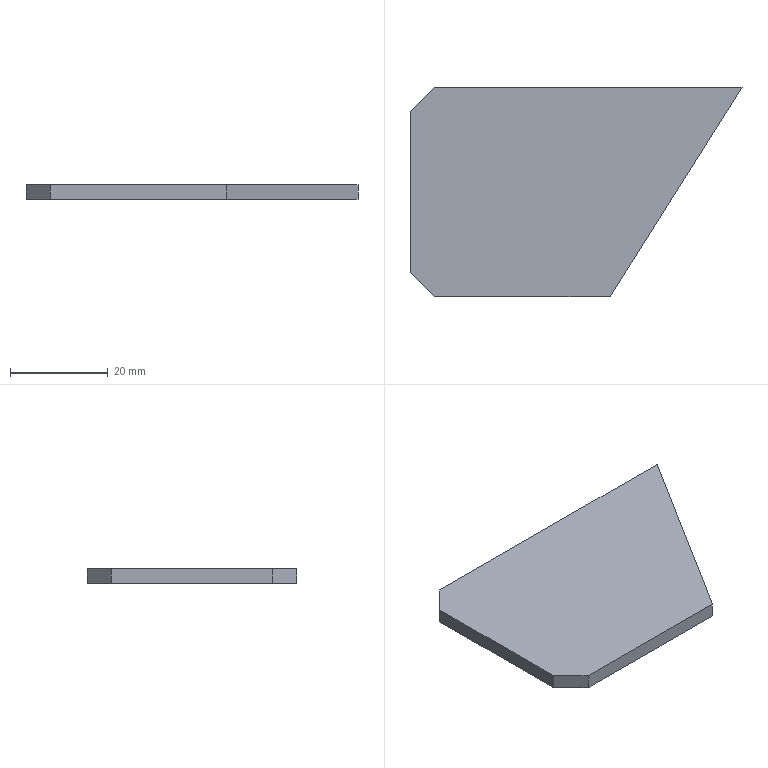Part | SolidWorks | features Chamfer 1, FlatPattern 1, ICE 1, SMBaseFlange 1, SheetMetal 1 | 1 solid | 8 faces | box 68 x 43 x 3 mm | volume 6956 mm3 | plane 8
STEP:
#1=CARTESIAN_POINT('',(68.,21.5,-3.));
#2=VERTEX_POINT('',#1);
#3=CARTESIAN_POINT('',(5.,21.5,-3.));
#4=VERTEX_POINT('',#3);
#5=CARTESIAN_POINT('',(68.,21.5,-3.));
#6=DIRECTION('',(-1.,0.,0.));
#7=VECTOR('',#6,1000.);
#8=LINE('',#5,#7);
#9=EDGE_CURVE('',#2,#4,#8,.T.);
#10=ORIENTED_EDGE('',*,*,#9,.T.);
#11=CARTESIAN_POINT('',(5.,21.5,0.));
#12=VERTEX_POINT('',#11);
#13=CARTESIAN_POINT('',(5.,21.5,-3.));
#14=DIRECTION('',(0.,0.,1.));
#15=VECTOR('',#14,1000.);
#16=LINE('',#13,#15);
#17=EDGE_CURVE('',#4,#12,#16,.T.);
#18=ORIENTED_EDGE('',*,*,#17,.T.);
#19=CARTESIAN_POINT('',(68.,21.5,0.));
#20=VERTEX_POINT('',#19);
#21=CARTESIAN_POINT('',(68.,21.5,0.));
#22=DIRECTION('',(-1.,0.,0.));
#23=VECTOR('',#22,1000.);
#24=LINE('',#21,#23);
#25=EDGE_CURVE('',#20,#12,#24,.T.);
#26=ORIENTED_EDGE('',*,*,#25,.F.);
#27=CARTESIAN_POINT('',(68.,21.5,-3.));
#28=DIRECTION('',(0.,0.,1.));
#29=VECTOR('',#28,1000.);
#30=LINE('',#27,#29);
#31=EDGE_CURVE('',#2,#20,#30,.T.);
#32=ORIENTED_EDGE('',*,*,#31,.F.);
#33=EDGE_LOOP('',(#10,#18,#26,#32));
#34=FACE_OUTER_BOUND('',#33,.T.);
#35=CARTESIAN_POINT('',(68.,21.5,-3.));
#36=DIRECTION('',(0.,1.,0.));
#37=DIRECTION('',(-1.,0.,0.));
#38=AXIS2_PLACEMENT_3D('',#35,#36,#37);
#39=PLANE('',#38);
#40=ADVANCED_FACE('',(#34),#39,.T.);
#41=CARTESIAN_POINT('',(41.,-21.5,0.));
#42=VERTEX_POINT('',#41);
#43=CARTESIAN_POINT('',(41.,-21.5,0.));
#44=DIRECTION('',(0.5318,0.8469,0.));
#45=VECTOR('',#44,1000.);
#46=LINE('',#43,#45);
#47=EDGE_CURVE('',#42,#20,#46,.T.);
#48=ORIENTED_EDGE('',*,*,#47,.F.);
#49=CARTESIAN_POINT('',(41.,-21.5,-3.));
#50=VERTEX_POINT('',#49);
#51=CARTESIAN_POINT('',(41.,-21.5,-3.));
#52=DIRECTION('',(0.,0.,1.));
#53=VECTOR('',#52,1000.);
#54=LINE('',#51,#53);
#55=EDGE_CURVE('',#50,#42,#54,.T.);
#56=ORIENTED_EDGE('',*,*,#55,.F.);
#57=CARTESIAN_POINT('',(41.,-21.5,-3.));
#58=DIRECTION('',(0.5318,0.8469,0.));
#59=VECTOR('',#58,1000.);
#60=LINE('',#57,#59);
#61=EDGE_CURVE('',#50,#2,#60,.T.);
#62=ORIENTED_EDGE('',*,*,#61,.T.);
#63=ORIENTED_EDGE('',*,*,#31,.T.);
#64=EDGE_LOOP('',(#48,#56,#62,#63));
#65=FACE_OUTER_BOUND('',#64,.T.);
#66=CARTESIAN_POINT('',(41.,-21.5,-3.));
#67=DIRECTION('',(0.8469,-0.5318,0.));
#68=DIRECTION('',(0.5318,0.8469,0.));
#69=AXIS2_PLACEMENT_3D('',#66,#67,#68);
#70=PLANE('',#69);
#71=ADVANCED_FACE('',(#65),#70,.T.);
#72=CARTESIAN_POINT('',(5.,-21.5,0.));
#73=VERTEX_POINT('',#72);
#74=CARTESIAN_POINT('',(0.,-21.5,0.));
#75=DIRECTION('',(1.,0.,0.));
#76=VECTOR('',#75,1000.);
#77=LINE('',#74,#76);
#78=EDGE_CURVE('',#73,#42,#77,.T.);
#79=ORIENTED_EDGE('',*,*,#78,.F.);
#80=CARTESIAN_POINT('',(5.,-21.5,-3.));
#81=VERTEX_POINT('',#80);
#82=CARTESIAN_POINT('',(5.,-21.5,-3.));
#83=DIRECTION('',(0.,0.,-1.));
#84=VECTOR('',#83,1000.);
#85=LINE('',#82,#84);
#86=EDGE_CURVE('',#73,#81,#85,.T.);
#87=ORIENTED_EDGE('',*,*,#86,.T.);
#88=CARTESIAN_POINT('',(0.,-21.5,-3.));
#89=DIRECTION('',(1.,0.,0.));
#90=VECTOR('',#89,1000.);
#91=LINE('',#88,#90);
#92=EDGE_CURVE('',#81,#50,#91,.T.);
#93=ORIENTED_EDGE('',*,*,#92,.T.);
#94=ORIENTED_EDGE('',*,*,#55,.T.);
#95=EDGE_LOOP('',(#79,#87,#93,#94));
#96=FACE_OUTER_BOUND('',#95,.T.);
#97=CARTESIAN_POINT('',(0.,-21.5,-3.));
#98=DIRECTION('',(0.,-1.,0.));
#99=DIRECTION('',(0.,0.,-1.));
#100=AXIS2_PLACEMENT_3D('',#97,#98,#99);
#101=PLANE('',#100);
#102=ADVANCED_FACE('',(#96),#101,.T.);
#103=CARTESIAN_POINT('',(0.,16.5,-3.));
#104=VERTEX_POINT('',#103);
#105=CARTESIAN_POINT('',(0.,-16.5,-3.));
#106=VERTEX_POINT('',#105);
#107=CARTESIAN_POINT('',(0.,21.5,-3.));
#108=DIRECTION('',(0.,-1.,0.));
#109=VECTOR('',#108,1000.);
#110=LINE('',#107,#109);
#111=EDGE_CURVE('',#104,#106,#110,.T.);
#112=ORIENTED_EDGE('',*,*,#111,.T.);
#113=CARTESIAN_POINT('',(0.,-16.5,0.));
#114=VERTEX_POINT('',#113);
#115=CARTESIAN_POINT('',(0.,-16.5,-3.));
#116=DIRECTION('',(0.,0.,1.));
#117=VECTOR('',#116,1000.);
#118=LINE('',#115,#117);
#119=EDGE_CURVE('',#106,#114,#118,.T.);
#120=ORIENTED_EDGE('',*,*,#119,.T.);
#121=CARTESIAN_POINT('',(0.,16.5,0.));
#122=VERTEX_POINT('',#121);
#123=CARTESIAN_POINT('',(0.,21.5,0.));
#124=DIRECTION('',(0.,-1.,0.));
#125=VECTOR('',#124,1000.);
#126=LINE('',#123,#125);
#127=EDGE_CURVE('',#122,#114,#126,.T.);
#128=ORIENTED_EDGE('',*,*,#127,.F.);
#129=CARTESIAN_POINT('',(0.,16.5,-3.));
#130=DIRECTION('',(0.,0.,-1.));
#131=VECTOR('',#130,1000.);
#132=LINE('',#129,#131);
#133=EDGE_CURVE('',#122,#104,#132,.T.);
#134=ORIENTED_EDGE('',*,*,#133,.T.);
#135=EDGE_LOOP('',(#112,#120,#128,#134));
#136=FACE_OUTER_BOUND('',#135,.T.);
#137=CARTESIAN_POINT('',(0.,21.5,-3.));
#138=DIRECTION('',(-1.,0.,0.));
#139=DIRECTION('',(0.,-1.,0.));
#140=AXIS2_PLACEMENT_3D('',#137,#138,#139);
#141=PLANE('',#140);
#142=ADVANCED_FACE('',(#136),#141,.T.);
#143=ORIENTED_EDGE('',*,*,#92,.F.);
#144=CARTESIAN_POINT('',(0.,-16.5,-3.));
#145=DIRECTION('',(-0.7071,0.7071,0.));
#146=VECTOR('',#145,1000.);
#147=LINE('',#144,#146);
#148=EDGE_CURVE('',#81,#106,#147,.T.);
#149=ORIENTED_EDGE('',*,*,#148,.T.);
#150=ORIENTED_EDGE('',*,*,#111,.F.);
#151=CARTESIAN_POINT('',(5.,21.5,-3.));
#152=DIRECTION('',(0.7071,0.7071,0.));
#153=VECTOR('',#152,1000.);
#154=LINE('',#151,#153);
#155=EDGE_CURVE('',#104,#4,#154,.T.);
#156=ORIENTED_EDGE('',*,*,#155,.T.);
#157=ORIENTED_EDGE('',*,*,#9,.F.);
#158=ORIENTED_EDGE('',*,*,#61,.F.);
#159=EDGE_LOOP('',(#143,#149,#150,#156,#157,#158));
#160=FACE_OUTER_BOUND('',#159,.T.);
#161=CARTESIAN_POINT('',(0.,0.,-3.));
#162=DIRECTION('',(0.,0.,1.));
#163=DIRECTION('',(1.,0.,0.));
#164=AXIS2_PLACEMENT_3D('',#161,#162,#163);
#165=PLANE('',#164);
#166=ADVANCED_FACE('',(#160),#165,.F.);
#167=ORIENTED_EDGE('',*,*,#127,.T.);
#168=CARTESIAN_POINT('',(-8.25,-8.25,0.));
#169=DIRECTION('',(0.7071,-0.7071,0.));
#170=VECTOR('',#169,1000.);
#171=LINE('',#168,#170);
#172=EDGE_CURVE('',#114,#73,#171,.T.);
#173=ORIENTED_EDGE('',*,*,#172,.T.);
#174=ORIENTED_EDGE('',*,*,#78,.T.);
#175=ORIENTED_EDGE('',*,*,#47,.T.);
#176=ORIENTED_EDGE('',*,*,#25,.T.);
#177=CARTESIAN_POINT('',(-8.25,8.25,0.));
#178=DIRECTION('',(-0.7071,-0.7071,0.));
#179=VECTOR('',#178,1000.);
#180=LINE('',#177,#179);
#181=EDGE_CURVE('',#12,#122,#180,.T.);
#182=ORIENTED_EDGE('',*,*,#181,.T.);
#183=EDGE_LOOP('',(#167,#173,#174,#175,#176,#182));
#184=FACE_OUTER_BOUND('',#183,.T.);
#185=CARTESIAN_POINT('',(0.,0.,0.));
#186=DIRECTION('',(0.,0.,1.));
#187=DIRECTION('',(1.,0.,0.));
#188=AXIS2_PLACEMENT_3D('',#185,#186,#187);
#189=PLANE('',#188);
#190=ADVANCED_FACE('',(#184),#189,.T.);
#191=ORIENTED_EDGE('',*,*,#148,.F.);
#192=ORIENTED_EDGE('',*,*,#86,.F.);
#193=ORIENTED_EDGE('',*,*,#172,.F.);
#194=ORIENTED_EDGE('',*,*,#119,.F.);
#195=EDGE_LOOP('',(#191,#192,#193,#194));
#196=FACE_OUTER_BOUND('',#195,.T.);
#197=CARTESIAN_POINT('',(0.,-16.5,-3.));
#198=DIRECTION('',(0.7071,0.7071,0.));
#199=DIRECTION('',(0.,0.,1.));
#200=AXIS2_PLACEMENT_3D('',#197,#198,#199);
#201=PLANE('',#200);
#202=ADVANCED_FACE('',(#196),#201,.F.);
#203=ORIENTED_EDGE('',*,*,#155,.F.);
#204=ORIENTED_EDGE('',*,*,#133,.F.);
#205=ORIENTED_EDGE('',*,*,#181,.F.);
#206=ORIENTED_EDGE('',*,*,#17,.F.);
#207=EDGE_LOOP('',(#203,#204,#205,#206));
#208=FACE_OUTER_BOUND('',#207,.T.);
#209=CARTESIAN_POINT('',(5.,21.5,-3.));
#210=DIRECTION('',(0.7071,-0.7071,0.));
#211=DIRECTION('',(0.,0.,1.));
#212=AXIS2_PLACEMENT_3D('',#209,#210,#211);
#213=PLANE('',#212);
#214=ADVANCED_FACE('',(#208),#213,.F.);
#215=CLOSED_SHELL('',(#40,#71,#102,#142,#166,#190,#202,#214));
#216=MANIFOLD_SOLID_BREP('',#215);
#217=CARTESIAN_POINT('',(0.,0.,0.));
#218=DIRECTION('',(0.,0.,1.));
#219=DIRECTION('',(1.,0.,0.));
#220=AXIS2_PLACEMENT_3D('',#217,#218,#219);
#221=(LENGTH_UNIT()NAMED_UNIT(*)SI_UNIT(.MILLI.,.METRE.));
#222=UNCERTAINTY_MEASURE_WITH_UNIT(LENGTH_MEASURE(0.00001),#221,'','');
#223=(NAMED_UNIT(*)PLANE_ANGLE_UNIT()SI_UNIT($,.RADIAN.));
#224=(NAMED_UNIT(*)SI_UNIT($,.STERADIAN.)SOLID_ANGLE_UNIT());
#225=(GEOMETRIC_REPRESENTATION_CONTEXT(3)GLOBAL_UNCERTAINTY_ASSIGNED_CONTEXT((#222))GLOBAL_UNIT_ASSIGNED_CONTEXT((#221,#223,#224))REPRESENTATION_CONTEXT('',''));
#226=ADVANCED_BREP_SHAPE_REPRESENTATION('',(#216,#220),#225);